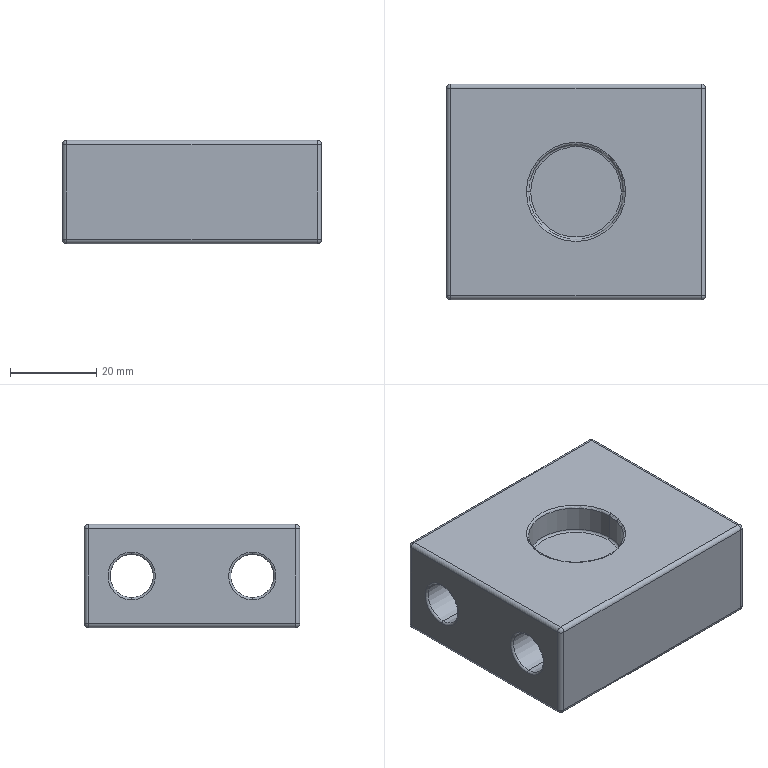Part | SolidWorks | features Fillet 2, ICE 2, Extrusion 1 | 1 solid | 45 faces | box 60 x 50 x 24 mm | volume 59794 mm3 | cylinder 18 | torus 12 | sphere 8 | plane 7 | commonest cylinder face diameters 2 x12 10 x4 22 x2
STEP:
#1=CARTESIAN_POINT('',(-29.5,14.,5.));
#2=VERTEX_POINT('',#1);
#3=CARTESIAN_POINT('',(-29.5,14.,-5.));
#4=VERTEX_POINT('',#3);
#5=CARTESIAN_POINT('',(-29.5,14.,0.));
#6=DIRECTION('',(-1.,0.,0.));
#7=DIRECTION('',(0.,0.,-1.));
#8=AXIS2_PLACEMENT_3D('',#5,#6,#7);
#9=CIRCLE('',#8,5.);
#10=EDGE_CURVE('',#2,#4,#9,.T.);
#11=ORIENTED_EDGE('',*,*,#10,.F.);
#12=CARTESIAN_POINT('',(-30.,14.,5.5));
#13=VERTEX_POINT('',#12);
#14=CARTESIAN_POINT('',(-29.5,14.,5.5));
#15=DIRECTION('',(0.,1.,0.));
#16=DIRECTION('',(0.,0.,1.));
#17=AXIS2_PLACEMENT_3D('',#14,#15,#16);
#18=CIRCLE('',#17,0.5);
#19=EDGE_CURVE('',#2,#13,#18,.T.);
#20=ORIENTED_EDGE('',*,*,#19,.T.);
#21=CARTESIAN_POINT('',(-30.,14.,-5.5));
#22=VERTEX_POINT('',#21);
#23=CARTESIAN_POINT('',(-30.,14.,0.));
#24=DIRECTION('',(1.,0.,0.));
#25=DIRECTION('',(0.,0.,-1.));
#26=AXIS2_PLACEMENT_3D('',#23,#24,#25);
#27=CIRCLE('',#26,5.5);
#28=EDGE_CURVE('',#22,#13,#27,.T.);
#29=ORIENTED_EDGE('',*,*,#28,.F.);
#30=CARTESIAN_POINT('',(-29.5,14.,-5.5));
#31=DIRECTION('',(0.,-1.,0.));
#32=DIRECTION('',(0.,0.,-1.));
#33=AXIS2_PLACEMENT_3D('',#30,#31,#32);
#34=CIRCLE('',#33,0.5);
#35=EDGE_CURVE('',#4,#22,#34,.T.);
#36=ORIENTED_EDGE('',*,*,#35,.F.);
#37=EDGE_LOOP('',(#11,#20,#29,#36));
#38=FACE_OUTER_BOUND('',#37,.T.);
#39=CARTESIAN_POINT('',(-29.5,14.,0.));
#40=DIRECTION('',(1.,0.,0.));
#41=DIRECTION('',(0.,0.,-1.));
#42=AXIS2_PLACEMENT_3D('',#39,#40,#41);
#43=TOROIDAL_SURFACE('',#42,5.5,0.5);
#44=ADVANCED_FACE('',(#38),#43,.T.);
#45=CARTESIAN_POINT('',(29.5,14.,-5.));
#46=VERTEX_POINT('',#45);
#47=CARTESIAN_POINT('',(29.5,14.,5.));
#48=VERTEX_POINT('',#47);
#49=CARTESIAN_POINT('',(29.5,14.,0.));
#50=DIRECTION('',(1.,0.,0.));
#51=DIRECTION('',(0.,0.,1.));
#52=AXIS2_PLACEMENT_3D('',#49,#50,#51);
#53=CIRCLE('',#52,5.);
#54=EDGE_CURVE('',#46,#48,#53,.T.);
#55=ORIENTED_EDGE('',*,*,#54,.F.);
#56=CARTESIAN_POINT('',(30.,14.,-5.5));
#57=VERTEX_POINT('',#56);
#58=CARTESIAN_POINT('',(29.5,14.,-5.5));
#59=DIRECTION('',(0.,1.,0.));
#60=DIRECTION('',(0.,0.,1.));
#61=AXIS2_PLACEMENT_3D('',#58,#59,#60);
#62=CIRCLE('',#61,0.5);
#63=EDGE_CURVE('',#46,#57,#62,.T.);
#64=ORIENTED_EDGE('',*,*,#63,.T.);
#65=CARTESIAN_POINT('',(30.,14.,5.5));
#66=VERTEX_POINT('',#65);
#67=CARTESIAN_POINT('',(30.,14.,0.));
#68=DIRECTION('',(-1.,0.,0.));
#69=DIRECTION('',(0.,0.,1.));
#70=AXIS2_PLACEMENT_3D('',#67,#68,#69);
#71=CIRCLE('',#70,5.5);
#72=EDGE_CURVE('',#66,#57,#71,.T.);
#73=ORIENTED_EDGE('',*,*,#72,.F.);
#74=CARTESIAN_POINT('',(29.5,14.,5.5));
#75=DIRECTION('',(0.,-1.,0.));
#76=DIRECTION('',(0.,0.,-1.));
#77=AXIS2_PLACEMENT_3D('',#74,#75,#76);
#78=CIRCLE('',#77,0.5);
#79=EDGE_CURVE('',#48,#66,#78,.T.);
#80=ORIENTED_EDGE('',*,*,#79,.F.);
#81=EDGE_LOOP('',(#55,#64,#73,#80));
#82=FACE_OUTER_BOUND('',#81,.T.);
#83=CARTESIAN_POINT('',(29.5,14.,0.));
#84=DIRECTION('',(-1.,0.,0.));
#85=DIRECTION('',(0.,0.,1.));
#86=AXIS2_PLACEMENT_3D('',#83,#84,#85);
#87=TOROIDAL_SURFACE('',#86,5.5,0.5);
#88=ADVANCED_FACE('',(#82),#87,.T.);
#89=CARTESIAN_POINT('',(-29.5,-14.,5.));
#90=VERTEX_POINT('',#89);
#91=CARTESIAN_POINT('',(-29.5,-14.,-5.));
#92=VERTEX_POINT('',#91);
#93=CARTESIAN_POINT('',(-29.5,-14.,0.));
#94=DIRECTION('',(-1.,0.,0.));
#95=DIRECTION('',(0.,0.,-1.));
#96=AXIS2_PLACEMENT_3D('',#93,#94,#95);
#97=CIRCLE('',#96,5.);
#98=EDGE_CURVE('',#90,#92,#97,.T.);
#99=ORIENTED_EDGE('',*,*,#98,.F.);
#100=CARTESIAN_POINT('',(-30.,-14.,5.5));
#101=VERTEX_POINT('',#100);
#102=CARTESIAN_POINT('',(-29.5,-14.,5.5));
#103=DIRECTION('',(0.,1.,0.));
#104=DIRECTION('',(0.,0.,1.));
#105=AXIS2_PLACEMENT_3D('',#102,#103,#104);
#106=CIRCLE('',#105,0.5);
#107=EDGE_CURVE('',#90,#101,#106,.T.);
#108=ORIENTED_EDGE('',*,*,#107,.T.);
#109=CARTESIAN_POINT('',(-30.,-14.,-5.5));
#110=VERTEX_POINT('',#109);
#111=CARTESIAN_POINT('',(-30.,-14.,0.));
#112=DIRECTION('',(1.,0.,0.));
#113=DIRECTION('',(0.,0.,-1.));
#114=AXIS2_PLACEMENT_3D('',#111,#112,#113);
#115=CIRCLE('',#114,5.5);
#116=EDGE_CURVE('',#110,#101,#115,.T.);
#117=ORIENTED_EDGE('',*,*,#116,.F.);
#118=CARTESIAN_POINT('',(-29.5,-14.,-5.5));
#119=DIRECTION('',(0.,-1.,0.));
#120=DIRECTION('',(0.,0.,-1.));
#121=AXIS2_PLACEMENT_3D('',#118,#119,#120);
#122=CIRCLE('',#121,0.5);
#123=EDGE_CURVE('',#92,#110,#122,.T.);
#124=ORIENTED_EDGE('',*,*,#123,.F.);
#125=EDGE_LOOP('',(#99,#108,#117,#124));
#126=FACE_OUTER_BOUND('',#125,.T.);
#127=CARTESIAN_POINT('',(-29.5,-14.,0.));
#128=DIRECTION('',(1.,0.,0.));
#129=DIRECTION('',(0.,0.,-1.));
#130=AXIS2_PLACEMENT_3D('',#127,#128,#129);
#131=TOROIDAL_SURFACE('',#130,5.5,0.5);
#132=ADVANCED_FACE('',(#126),#131,.T.);
#133=CARTESIAN_POINT('',(29.5,-14.,-5.));
#134=VERTEX_POINT('',#133);
#135=CARTESIAN_POINT('',(29.5,-14.,5.));
#136=VERTEX_POINT('',#135);
#137=CARTESIAN_POINT('',(29.5,-14.,0.));
#138=DIRECTION('',(1.,0.,0.));
#139=DIRECTION('',(0.,0.,1.));
#140=AXIS2_PLACEMENT_3D('',#137,#138,#139);
#141=CIRCLE('',#140,5.);
#142=EDGE_CURVE('',#134,#136,#141,.T.);
#143=ORIENTED_EDGE('',*,*,#142,.F.);
#144=CARTESIAN_POINT('',(30.,-14.,-5.5));
#145=VERTEX_POINT('',#144);
#146=CARTESIAN_POINT('',(29.5,-14.,-5.5));
#147=DIRECTION('',(0.,1.,0.));
#148=DIRECTION('',(0.,0.,1.));
#149=AXIS2_PLACEMENT_3D('',#146,#147,#148);
#150=CIRCLE('',#149,0.5);
#151=EDGE_CURVE('',#134,#145,#150,.T.);
#152=ORIENTED_EDGE('',*,*,#151,.T.);
#153=CARTESIAN_POINT('',(30.,-14.,5.5));
#154=VERTEX_POINT('',#153);
#155=CARTESIAN_POINT('',(30.,-14.,0.));
#156=DIRECTION('',(-1.,0.,0.));
#157=DIRECTION('',(0.,0.,1.));
#158=AXIS2_PLACEMENT_3D('',#155,#156,#157);
#159=CIRCLE('',#158,5.5);
#160=EDGE_CURVE('',#154,#145,#159,.T.);
#161=ORIENTED_EDGE('',*,*,#160,.F.);
#162=CARTESIAN_POINT('',(29.5,-14.,5.5));
#163=DIRECTION('',(0.,-1.,0.));
#164=DIRECTION('',(0.,0.,-1.));
#165=AXIS2_PLACEMENT_3D('',#162,#163,#164);
#166=CIRCLE('',#165,0.5);
#167=EDGE_CURVE('',#136,#154,#166,.T.);
#168=ORIENTED_EDGE('',*,*,#167,.F.);
#169=EDGE_LOOP('',(#143,#152,#161,#168));
#170=FACE_OUTER_BOUND('',#169,.T.);
#171=CARTESIAN_POINT('',(29.5,-14.,0.));
#172=DIRECTION('',(-1.,0.,0.));
#173=DIRECTION('',(0.,0.,1.));
#174=AXIS2_PLACEMENT_3D('',#171,#172,#173);
#175=TOROIDAL_SURFACE('',#174,5.5,0.5);
#176=ADVANCED_FACE('',(#170),#175,.T.);
#177=CARTESIAN_POINT('',(-10.5,0.,5.));
#178=VERTEX_POINT('',#177);
#179=CARTESIAN_POINT('',(10.5,0.,5.));
#180=VERTEX_POINT('',#179);
#181=CARTESIAN_POINT('',(0.,0.,5.));
#182=DIRECTION('',(0.,0.,1.));
#183=DIRECTION('',(1.,0.,0.));
#184=AXIS2_PLACEMENT_3D('',#181,#182,#183);
#185=CIRCLE('',#184,10.5);
#186=EDGE_CURVE('',#178,#180,#185,.T.);
#187=ORIENTED_EDGE('',*,*,#186,.F.);
#188=CARTESIAN_POINT('',(-11.,0.,5.5));
#189=VERTEX_POINT('',#188);
#190=CARTESIAN_POINT('',(-10.5,0.,5.5));
#191=DIRECTION('',(0.,1.,0.));
#192=DIRECTION('',(-1.,0.,0.));
#193=AXIS2_PLACEMENT_3D('',#190,#191,#192);
#194=CIRCLE('',#193,0.5);
#195=EDGE_CURVE('',#178,#189,#194,.T.);
#196=ORIENTED_EDGE('',*,*,#195,.T.);
#197=CARTESIAN_POINT('',(11.,0.,5.5));
#198=VERTEX_POINT('',#197);
#199=CARTESIAN_POINT('',(0.,0.,5.5));
#200=DIRECTION('',(0.,0.,-1.));
#201=DIRECTION('',(1.,0.,0.));
#202=AXIS2_PLACEMENT_3D('',#199,#200,#201);
#203=CIRCLE('',#202,11.);
#204=EDGE_CURVE('',#198,#189,#203,.T.);
#205=ORIENTED_EDGE('',*,*,#204,.F.);
#206=CARTESIAN_POINT('',(10.5,0.,5.5));
#207=DIRECTION('',(0.,-1.,0.));
#208=DIRECTION('',(0.,0.,-1.));
#209=AXIS2_PLACEMENT_3D('',#206,#207,#208);
#210=CIRCLE('',#209,0.5);
#211=EDGE_CURVE('',#180,#198,#210,.T.);
#212=ORIENTED_EDGE('',*,*,#211,.F.);
#213=EDGE_LOOP('',(#187,#196,#205,#212));
#214=FACE_OUTER_BOUND('',#213,.T.);
#215=CARTESIAN_POINT('',(0.,0.,5.5));
#216=DIRECTION('',(0.,0.,1.));
#217=DIRECTION('',(1.,0.,0.));
#218=AXIS2_PLACEMENT_3D('',#215,#216,#217);
#219=TOROIDAL_SURFACE('',#218,10.5,0.5);
#220=ADVANCED_FACE('',(#214),#219,.F.);
#221=CARTESIAN_POINT('',(-11.5,0.,12.));
#222=VERTEX_POINT('',#221);
#223=CARTESIAN_POINT('',(11.5,0.,12.));
#224=VERTEX_POINT('',#223);
#225=CARTESIAN_POINT('',(0.,0.,12.));
#226=DIRECTION('',(0.,0.,-1.));
#227=DIRECTION('',(1.,0.,0.));
#228=AXIS2_PLACEMENT_3D('',#225,#226,#227);
#229=CIRCLE('',#228,11.5);
#230=EDGE_CURVE('',#222,#224,#229,.T.);
#231=ORIENTED_EDGE('',*,*,#230,.F.);
#232=CARTESIAN_POINT('',(-11.,0.,11.5));
#233=VERTEX_POINT('',#232);
#234=CARTESIAN_POINT('',(-11.5,0.,11.5));
#235=DIRECTION('',(0.,1.,0.));
#236=DIRECTION('',(-1.,0.,0.));
#237=AXIS2_PLACEMENT_3D('',#234,#235,#236);
#238=CIRCLE('',#237,0.5);
#239=EDGE_CURVE('',#222,#233,#238,.T.);
#240=ORIENTED_EDGE('',*,*,#239,.T.);
#241=CARTESIAN_POINT('',(11.,0.,11.5));
#242=VERTEX_POINT('',#241);
#243=CARTESIAN_POINT('',(0.,0.,11.5));
#244=DIRECTION('',(0.,0.,1.));
#245=DIRECTION('',(1.,0.,0.));
#246=AXIS2_PLACEMENT_3D('',#243,#244,#245);
#247=CIRCLE('',#246,11.);
#248=EDGE_CURVE('',#242,#233,#247,.T.);
#249=ORIENTED_EDGE('',*,*,#248,.F.);
#250=CARTESIAN_POINT('',(11.5,0.,11.5));
#251=DIRECTION('',(0.,-1.,0.));
#252=DIRECTION('',(0.,0.,-1.));
#253=AXIS2_PLACEMENT_3D('',#250,#251,#252);
#254=CIRCLE('',#253,0.5);
#255=EDGE_CURVE('',#224,#242,#254,.T.);
#256=ORIENTED_EDGE('',*,*,#255,.F.);
#257=EDGE_LOOP('',(#231,#240,#249,#256));
#258=FACE_OUTER_BOUND('',#257,.T.);
#259=CARTESIAN_POINT('',(0.,0.,11.5));
#260=DIRECTION('',(0.,0.,1.));
#261=DIRECTION('',(1.,0.,0.));
#262=AXIS2_PLACEMENT_3D('',#259,#260,#261);
#263=TOROIDAL_SURFACE('',#262,11.5,0.5);
#264=ADVANCED_FACE('',(#258),#263,.T.);
#265=CARTESIAN_POINT('',(-29.5,-14.,0.));
#266=DIRECTION('',(-1.,0.,0.));
#267=DIRECTION('',(0.,0.,-1.));
#268=AXIS2_PLACEMENT_3D('',#265,#266,#267);
#269=CIRCLE('',#268,5.);
#270=EDGE_CURVE('',#92,#90,#269,.T.);
#271=ORIENTED_EDGE('',*,*,#270,.T.);
#272=CARTESIAN_POINT('',(-30.,-14.,5.));
#273=DIRECTION('',(1.,0.,0.));
#274=VECTOR('',#273,1000.);
#275=LINE('',#272,#274);
#276=EDGE_CURVE('',#90,#136,#275,.T.);
#277=ORIENTED_EDGE('',*,*,#276,.T.);
#278=CARTESIAN_POINT('',(29.5,-14.,0.));
#279=DIRECTION('',(1.,0.,0.));
#280=DIRECTION('',(0.,0.,1.));
#281=AXIS2_PLACEMENT_3D('',#278,#279,#280);
#282=CIRCLE('',#281,5.);
#283=EDGE_CURVE('',#136,#134,#282,.T.);
#284=ORIENTED_EDGE('',*,*,#283,.T.);
#285=CARTESIAN_POINT('',(-30.,-14.,-5.));
#286=DIRECTION('',(1.,0.,0.));
#287=VECTOR('',#286,1000.);
#288=LINE('',#285,#287);
#289=EDGE_CURVE('',#92,#134,#288,.T.);
#290=ORIENTED_EDGE('',*,*,#289,.F.);
#291=EDGE_LOOP('',(#271,#277,#284,#290));
#292=FACE_OUTER_BOUND('',#291,.T.);
#293=CARTESIAN_POINT('',(-30.,-14.,0.));
#294=DIRECTION('',(1.,0.,0.));
#295=DIRECTION('',(0.,0.,-1.));
#296=AXIS2_PLACEMENT_3D('',#293,#294,#295);
#297=CYLINDRICAL_SURFACE('',#296,5.);
#298=ADVANCED_FACE('',(#292),#297,.F.);
#299=CARTESIAN_POINT('',(-29.5,14.,0.));
#300=DIRECTION('',(-1.,0.,0.));
#301=DIRECTION('',(0.,0.,-1.));
#302=AXIS2_PLACEMENT_3D('',#299,#300,#301);
#303=CIRCLE('',#302,5.);
#304=EDGE_CURVE('',#4,#2,#303,.T.);
#305=ORIENTED_EDGE('',*,*,#304,.T.);
#306=CARTESIAN_POINT('',(-30.,14.,5.));
#307=DIRECTION('',(1.,0.,0.));
#308=VECTOR('',#307,1000.);
#309=LINE('',#306,#308);
#310=EDGE_CURVE('',#2,#48,#309,.T.);
#311=ORIENTED_EDGE('',*,*,#310,.T.);
#312=CARTESIAN_POINT('',(29.5,14.,0.));
#313=DIRECTION('',(1.,0.,0.));
#314=DIRECTION('',(0.,0.,1.));
#315=AXIS2_PLACEMENT_3D('',#312,#313,#314);
#316=CIRCLE('',#315,5.);
#317=EDGE_CURVE('',#48,#46,#316,.T.);
#318=ORIENTED_EDGE('',*,*,#317,.T.);
#319=CARTESIAN_POINT('',(-30.,14.,-5.));
#320=DIRECTION('',(1.,0.,0.));
#321=VECTOR('',#320,1000.);
#322=LINE('',#319,#321);
#323=EDGE_CURVE('',#4,#46,#322,.T.);
#324=ORIENTED_EDGE('',*,*,#323,.F.);
#325=EDGE_LOOP('',(#305,#311,#318,#324));
#326=FACE_OUTER_BOUND('',#325,.T.);
#327=CARTESIAN_POINT('',(-30.,14.,0.));
#328=DIRECTION('',(1.,0.,0.));
#329=DIRECTION('',(0.,0.,-1.));
#330=AXIS2_PLACEMENT_3D('',#327,#328,#329);
#331=CYLINDRICAL_SURFACE('',#330,5.);
#332=ADVANCED_FACE('',(#326),#331,.F.);
#333=ORIENTED_EDGE('',*,*,#204,.T.);
#334=CARTESIAN_POINT('',(-11.,0.,5.));
#335=DIRECTION('',(0.,0.,1.));
#336=VECTOR('',#335,1000.);
#337=LINE('',#334,#336);
#338=EDGE_CURVE('',#189,#233,#337,.T.);
#339=ORIENTED_EDGE('',*,*,#338,.T.);
#340=CARTESIAN_POINT('',(0.,0.,11.5));
#341=DIRECTION('',(0.,0.,1.));
#342=DIRECTION('',(1.,0.,0.));
#343=AXIS2_PLACEMENT_3D('',#340,#341,#342);
#344=CIRCLE('',#343,11.);
#345=EDGE_CURVE('',#233,#242,#344,.T.);
#346=ORIENTED_EDGE('',*,*,#345,.T.);
#347=CARTESIAN_POINT('',(11.,0.,5.));
#348=DIRECTION('',(0.,0.,1.));
#349=VECTOR('',#348,1000.);
#350=LINE('',#347,#349);
#351=EDGE_CURVE('',#198,#242,#350,.T.);
#352=ORIENTED_EDGE('',*,*,#351,.F.);
#353=EDGE_LOOP('',(#333,#339,#346,#352));
#354=FACE_OUTER_BOUND('',#353,.T.);
#355=CARTESIAN_POINT('',(0.,0.,5.));
#356=DIRECTION('',(0.,0.,1.));
#357=DIRECTION('',(1.,0.,0.));
#358=AXIS2_PLACEMENT_3D('',#355,#356,#357);
#359=CYLINDRICAL_SURFACE('',#358,11.);
#360=ADVANCED_FACE('',(#354),#359,.F.);
#361=ORIENTED_EDGE('',*,*,#116,.T.);
#362=CARTESIAN_POINT('',(-30.,-14.,0.));
#363=DIRECTION('',(1.,0.,0.));
#364=DIRECTION('',(0.,0.,-1.));
#365=AXIS2_PLACEMENT_3D('',#362,#363,#364);
#366=CIRCLE('',#365,5.5);
#367=EDGE_CURVE('',#101,#110,#366,.T.);
#368=ORIENTED_EDGE('',*,*,#367,.T.);
#369=EDGE_LOOP('',(#361,#368));
#370=FACE_BOUND('',#369,.T.);
#371=ORIENTED_EDGE('',*,*,#28,.T.);
#372=CARTESIAN_POINT('',(-30.,14.,0.));
#373=DIRECTION('',(1.,0.,0.));
#374=DIRECTION('',(0.,0.,-1.));
#375=AXIS2_PLACEMENT_3D('',#372,#373,#374);
#376=CIRCLE('',#375,5.5);
#377=EDGE_CURVE('',#13,#22,#376,.T.);
#378=ORIENTED_EDGE('',*,*,#377,.T.);
#379=EDGE_LOOP('',(#371,#378));
#380=FACE_BOUND('',#379,.T.);
#381=CARTESIAN_POINT('',(-30.,24.,11.));
#382=VERTEX_POINT('',#381);
#383=CARTESIAN_POINT('',(-30.,24.,-11.));
#384=VERTEX_POINT('',#383);
#385=CARTESIAN_POINT('',(-30.,24.,12.));
#386=DIRECTION('',(0.,0.,-1.));
#387=VECTOR('',#386,1000.);
#388=LINE('',#385,#387);
#389=EDGE_CURVE('',#382,#384,#388,.T.);
#390=ORIENTED_EDGE('',*,*,#389,.T.);
#391=CARTESIAN_POINT('',(-30.,-24.,-11.));
#392=VERTEX_POINT('',#391);
#393=CARTESIAN_POINT('',(-30.,-25.,-11.));
#394=DIRECTION('',(0.,-1.,0.));
#395=VECTOR('',#394,1000.);
#396=LINE('',#393,#395);
#397=EDGE_CURVE('',#384,#392,#396,.T.);
#398=ORIENTED_EDGE('',*,*,#397,.T.);
#399=CARTESIAN_POINT('',(-30.,-24.,11.));
#400=VERTEX_POINT('',#399);
#401=CARTESIAN_POINT('',(-30.,-24.,12.));
#402=DIRECTION('',(0.,0.,1.));
#403=VECTOR('',#402,1000.);
#404=LINE('',#401,#403);
#405=EDGE_CURVE('',#392,#400,#404,.T.);
#406=ORIENTED_EDGE('',*,*,#405,.T.);
#407=CARTESIAN_POINT('',(-30.,25.,11.));
#408=DIRECTION('',(0.,1.,0.));
#409=VECTOR('',#408,1000.);
#410=LINE('',#407,#409);
#411=EDGE_CURVE('',#400,#382,#410,.T.);
#412=ORIENTED_EDGE('',*,*,#411,.T.);
#413=EDGE_LOOP('',(#390,#398,#406,#412));
#414=FACE_OUTER_BOUND('',#413,.T.);
#415=CARTESIAN_POINT('',(-30.,-25.,12.));
#416=DIRECTION('',(1.,0.,0.));
#417=DIRECTION('',(0.,0.,-1.));
#418=AXIS2_PLACEMENT_3D('',#415,#416,#417);
#419=PLANE('',#418);
#420=ADVANCED_FACE('',(#370,#380,#414),#419,.F.);
#421=CARTESIAN_POINT('',(29.,-25.,11.));
#422=VERTEX_POINT('',#421);
#423=CARTESIAN_POINT('',(-29.,-25.,11.));
#424=VERTEX_POINT('',#423);
#425=CARTESIAN_POINT('',(-30.,-25.,11.));
#426=DIRECTION('',(-1.,0.,0.));
#427=VECTOR('',#426,1000.);
#428=LINE('',#425,#427);
#429=EDGE_CURVE('',#422,#424,#428,.T.);
#430=ORIENTED_EDGE('',*,*,#429,.T.);
#431=CARTESIAN_POINT('',(-29.,-25.,-11.));
#432=VERTEX_POINT('',#431);
#433=CARTESIAN_POINT('',(-29.,-25.,12.));
#434=DIRECTION('',(0.,0.,-1.));
#435=VECTOR('',#434,1000.);
#436=LINE('',#433,#435);
#437=EDGE_CURVE('',#424,#432,#436,.T.);
#438=ORIENTED_EDGE('',*,*,#437,.T.);
#439=CARTESIAN_POINT('',(29.,-25.,-11.));
#440=VERTEX_POINT('',#439);
#441=CARTESIAN_POINT('',(30.,-25.,-11.));
#442=DIRECTION('',(1.,0.,0.));
#443=VECTOR('',#442,1000.);
#444=LINE('',#441,#443);
#445=EDGE_CURVE('',#432,#440,#444,.T.);
#446=ORIENTED_EDGE('',*,*,#445,.T.);
#447=CARTESIAN_POINT('',(29.,-25.,12.));
#448=DIRECTION('',(0.,0.,1.));
#449=VECTOR('',#448,1000.);
#450=LINE('',#447,#449);
#451=EDGE_CURVE('',#440,#422,#450,.T.);
#452=ORIENTED_EDGE('',*,*,#451,.T.);
#453=EDGE_LOOP('',(#430,#438,#446,#452));
#454=FACE_OUTER_BOUND('',#453,.T.);
#455=CARTESIAN_POINT('',(30.,-25.,12.));
#456=DIRECTION('',(0.,1.,0.));
#457=DIRECTION('',(-1.,0.,0.));
#458=AXIS2_PLACEMENT_3D('',#455,#456,#457);
#459=PLANE('',#458);
#460=ADVANCED_FACE('',(#454),#459,.F.);
#461=ORIENTED_EDGE('',*,*,#160,.T.);
#462=CARTESIAN_POINT('',(30.,-14.,0.));
#463=DIRECTION('',(-1.,0.,0.));
#464=DIRECTION('',(0.,0.,1.));
#465=AXIS2_PLACEMENT_3D('',#462,#463,#464);
#466=CIRCLE('',#465,5.5);
#467=EDGE_CURVE('',#145,#154,#466,.T.);
#468=ORIENTED_EDGE('',*,*,#467,.T.);
#469=EDGE_LOOP('',(#461,#468));
#470=FACE_BOUND('',#469,.T.);
#471=ORIENTED_EDGE('',*,*,#72,.T.);
#472=CARTESIAN_POINT('',(30.,14.,0.));
#473=DIRECTION('',(-1.,0.,0.));
#474=DIRECTION('',(0.,0.,1.));
#475=AXIS2_PLACEMENT_3D('',#472,#473,#474);
#476=CIRCLE('',#475,5.5);
#477=EDGE_CURVE('',#57,#66,#476,.T.);
#478=ORIENTED_EDGE('',*,*,#477,.T.);
#479=EDGE_LOOP('',(#471,#478));
#480=FACE_BOUND('',#479,.T.);
#481=CARTESIAN_POINT('',(30.,-24.,11.));
#482=VERTEX_POINT('',#481);
#483=CARTESIAN_POINT('',(30.,-24.,-11.));
#484=VERTEX_POINT('',#483);
#485=CARTESIAN_POINT('',(30.,-24.,12.));
#486=DIRECTION('',(0.,0.,-1.));
#487=VECTOR('',#486,1000.);
#488=LINE('',#485,#487);
#489=EDGE_CURVE('',#482,#484,#488,.T.);
#490=ORIENTED_EDGE('',*,*,#489,.T.);
#491=CARTESIAN_POINT('',(30.,24.,-11.));
#492=VERTEX_POINT('',#491);
#493=CARTESIAN_POINT('',(30.,-25.,-11.));
#494=DIRECTION('',(0.,1.,0.));
#495=VECTOR('',#494,1000.);
#496=LINE('',#493,#495);
#497=EDGE_CURVE('',#484,#492,#496,.T.);
#498=ORIENTED_EDGE('',*,*,#497,.T.);
#499=CARTESIAN_POINT('',(30.,24.,11.));
#500=VERTEX_POINT('',#499);
#501=CARTESIAN_POINT('',(30.,24.,12.));
#502=DIRECTION('',(0.,0.,1.));
#503=VECTOR('',#502,1000.);
#504=LINE('',#501,#503);
#505=EDGE_CURVE('',#492,#500,#504,.T.);
#506=ORIENTED_EDGE('',*,*,#505,.T.);
#507=CARTESIAN_POINT('',(30.,-25.,11.));
#508=DIRECTION('',(0.,-1.,0.));
#509=VECTOR('',#508,1000.);
#510=LINE('',#507,#509);
#511=EDGE_CURVE('',#500,#482,#510,.T.);
#512=ORIENTED_EDGE('',*,*,#511,.T.);
#513=EDGE_LOOP('',(#490,#498,#506,#512));
#514=FACE_OUTER_BOUND('',#513,.T.);
#515=CARTESIAN_POINT('',(30.,-25.,12.));
#516=DIRECTION('',(-1.,0.,0.));
#517=DIRECTION('',(0.,0.,1.));
#518=AXIS2_PLACEMENT_3D('',#515,#516,#517);
#519=PLANE('',#518);
#520=ADVANCED_FACE('',(#470,#480,#514),#519,.F.);
#521=CARTESIAN_POINT('',(-29.,25.,11.));
#522=VERTEX_POINT('',#521);
#523=CARTESIAN_POINT('',(29.,25.,11.));
#524=VERTEX_POINT('',#523);
#525=CARTESIAN_POINT('',(30.,25.,11.));
#526=DIRECTION('',(1.,0.,0.));
#527=VECTOR('',#526,1000.);
#528=LINE('',#525,#527);
#529=EDGE_CURVE('',#522,#524,#528,.T.);
#530=ORIENTED_EDGE('',*,*,#529,.T.);
#531=CARTESIAN_POINT('',(29.,25.,-11.));
#532=VERTEX_POINT('',#531);
#533=CARTESIAN_POINT('',(29.,25.,12.));
#534=DIRECTION('',(0.,0.,-1.));
#535=VECTOR('',#534,1000.);
#536=LINE('',#533,#535);
#537=EDGE_CURVE('',#524,#532,#536,.T.);
#538=ORIENTED_EDGE('',*,*,#537,.T.);
#539=CARTESIAN_POINT('',(-29.,25.,-11.));
#540=VERTEX_POINT('',#539);
#541=CARTESIAN_POINT('',(30.,25.,-11.));
#542=DIRECTION('',(-1.,0.,0.));
#543=VECTOR('',#542,1000.);
#544=LINE('',#541,#543);
#545=EDGE_CURVE('',#532,#540,#544,.T.);
#546=ORIENTED_EDGE('',*,*,#545,.T.);
#547=CARTESIAN_POINT('',(-29.,25.,12.));
#548=DIRECTION('',(0.,0.,1.));
#549=VECTOR('',#548,1000.);
#550=LINE('',#547,#549);
#551=EDGE_CURVE('',#540,#522,#550,.T.);
#552=ORIENTED_EDGE('',*,*,#551,.T.);
#553=EDGE_LOOP('',(#530,#538,#546,#552));
#554=FACE_OUTER_BOUND('',#553,.T.);
#555=CARTESIAN_POINT('',(30.,25.,12.));
#556=DIRECTION('',(0.,-1.,0.));
#557=DIRECTION('',(1.,0.,0.));
#558=AXIS2_PLACEMENT_3D('',#555,#556,#557);
#559=PLANE('',#558);
#560=ADVANCED_FACE('',(#554),#559,.F.);
#561=CARTESIAN_POINT('',(0.,0.,12.));
#562=DIRECTION('',(0.,0.,-1.));
#563=DIRECTION('',(1.,0.,0.));
#564=AXIS2_PLACEMENT_3D('',#561,#562,#563);
#565=CIRCLE('',#564,11.5);
#566=EDGE_CURVE('',#224,#222,#565,.T.);
#567=ORIENTED_EDGE('',*,*,#566,.T.);
#568=ORIENTED_EDGE('',*,*,#230,.T.);
#569=EDGE_LOOP('',(#567,#568));
#570=FACE_BOUND('',#569,.T.);
#571=CARTESIAN_POINT('',(29.,24.,12.));
#572=VERTEX_POINT('',#571);
#573=CARTESIAN_POINT('',(-29.,24.,12.));
#574=VERTEX_POINT('',#573);
#575=CARTESIAN_POINT('',(-30.,24.,12.));
#576=DIRECTION('',(-1.,0.,0.));
#577=VECTOR('',#576,1000.);
#578=LINE('',#575,#577);
#579=EDGE_CURVE('',#572,#574,#578,.T.);
#580=ORIENTED_EDGE('',*,*,#579,.T.);
#581=CARTESIAN_POINT('',(-29.,-24.,12.));
#582=VERTEX_POINT('',#581);
#583=CARTESIAN_POINT('',(-29.,-25.,12.));
#584=DIRECTION('',(0.,-1.,0.));
#585=VECTOR('',#584,1000.);
#586=LINE('',#583,#585);
#587=EDGE_CURVE('',#574,#582,#586,.T.);
#588=ORIENTED_EDGE('',*,*,#587,.T.);
#589=CARTESIAN_POINT('',(29.,-24.,12.));
#590=VERTEX_POINT('',#589);
#591=CARTESIAN_POINT('',(30.,-24.,12.));
#592=DIRECTION('',(1.,0.,0.));
#593=VECTOR('',#592,1000.);
#594=LINE('',#591,#593);
#595=EDGE_CURVE('',#582,#590,#594,.T.);
#596=ORIENTED_EDGE('',*,*,#595,.T.);
#597=CARTESIAN_POINT('',(29.,25.,12.));
#598=DIRECTION('',(0.,1.,0.));
#599=VECTOR('',#598,1000.);
#600=LINE('',#597,#599);
#601=EDGE_CURVE('',#590,#572,#600,.T.);
#602=ORIENTED_EDGE('',*,*,#601,.T.);
#603=EDGE_LOOP('',(#580,#588,#596,#602));
#604=FACE_OUTER_BOUND('',#603,.T.);
#605=CARTESIAN_POINT('',(0.,0.,12.));
#606=DIRECTION('',(0.,0.,1.));
#607=DIRECTION('',(1.,0.,0.));
#608=AXIS2_PLACEMENT_3D('',#605,#606,#607);
#609=PLANE('',#608);
#610=ADVANCED_FACE('',(#570,#604),#609,.T.);
#611=CARTESIAN_POINT('',(29.,-24.,-12.));
#612=VERTEX_POINT('',#611);
#613=CARTESIAN_POINT('',(-29.,-24.,-12.));
#614=VERTEX_POINT('',#613);
#615=CARTESIAN_POINT('',(0.,-24.,-12.));
#616=DIRECTION('',(-1.,0.,0.));
#617=VECTOR('',#616,1000.);
#618=LINE('',#615,#617);
#619=EDGE_CURVE('',#612,#614,#618,.T.);
#620=ORIENTED_EDGE('',*,*,#619,.T.);
#621=CARTESIAN_POINT('',(-29.,24.,-12.));
#622=VERTEX_POINT('',#621);
#623=CARTESIAN_POINT('',(-29.,0.,-12.));
#624=DIRECTION('',(0.,1.,0.));
#625=VECTOR('',#624,1000.);
#626=LINE('',#623,#625);
#627=EDGE_CURVE('',#614,#622,#626,.T.);
#628=ORIENTED_EDGE('',*,*,#627,.T.);
#629=CARTESIAN_POINT('',(29.,24.,-12.));
#630=VERTEX_POINT('',#629);
#631=CARTESIAN_POINT('',(0.,24.,-12.));
#632=DIRECTION('',(1.,0.,0.));
#633=VECTOR('',#632,1000.);
#634=LINE('',#631,#633);
#635=EDGE_CURVE('',#622,#630,#634,.T.);
#636=ORIENTED_EDGE('',*,*,#635,.T.);
#637=CARTESIAN_POINT('',(29.,0.,-12.));
#638=DIRECTION('',(0.,-1.,0.));
#639=VECTOR('',#638,1000.);
#640=LINE('',#637,#639);
#641=EDGE_CURVE('',#630,#612,#640,.T.);
#642=ORIENTED_EDGE('',*,*,#641,.T.);
#643=EDGE_LOOP('',(#620,#628,#636,#642));
#644=FACE_OUTER_BOUND('',#643,.T.);
#645=CARTESIAN_POINT('',(0.,0.,-12.));
#646=DIRECTION('',(0.,0.,1.));
#647=DIRECTION('',(1.,0.,0.));
#648=AXIS2_PLACEMENT_3D('',#645,#646,#647);
#649=PLANE('',#648);
#650=ADVANCED_FACE('',(#644),#649,.F.);
#651=ORIENTED_EDGE('',*,*,#338,.F.);
#652=CARTESIAN_POINT('',(0.,0.,5.5));
#653=DIRECTION('',(0.,0.,-1.));
#654=DIRECTION('',(1.,0.,0.));
#655=AXIS2_PLACEMENT_3D('',#652,#653,#654);
#656=CIRCLE('',#655,11.);
#657=EDGE_CURVE('',#189,#198,#656,.T.);
#658=ORIENTED_EDGE('',*,*,#657,.T.);
#659=ORIENTED_EDGE('',*,*,#351,.T.);
#660=ORIENTED_EDGE('',*,*,#248,.T.);
#661=EDGE_LOOP('',(#651,#658,#659,#660));
#662=FACE_OUTER_BOUND('',#661,.T.);
#663=CARTESIAN_POINT('',(0.,0.,5.));
#664=DIRECTION('',(0.,0.,1.));
#665=DIRECTION('',(1.,0.,0.));
#666=AXIS2_PLACEMENT_3D('',#663,#664,#665);
#667=CYLINDRICAL_SURFACE('',#666,11.);
#668=ADVANCED_FACE('',(#662),#667,.F.);
#669=CARTESIAN_POINT('',(0.,0.,5.));
#670=DIRECTION('',(0.,0.,1.));
#671=DIRECTION('',(1.,0.,0.));
#672=AXIS2_PLACEMENT_3D('',#669,#670,#671);
#673=CIRCLE('',#672,10.5);
#674=EDGE_CURVE('',#180,#178,#673,.T.);
#675=ORIENTED_EDGE('',*,*,#674,.T.);
#676=ORIENTED_EDGE('',*,*,#186,.T.);
#677=EDGE_LOOP('',(#675,#676));
#678=FACE_OUTER_BOUND('',#677,.T.);
#679=CARTESIAN_POINT('',(0.,0.,5.));
#680=DIRECTION('',(0.,0.,1.));
#681=DIRECTION('',(1.,0.,0.));
#682=AXIS2_PLACEMENT_3D('',#679,#680,#681);
#683=PLANE('',#682);
#684=ADVANCED_FACE('',(#678),#683,.T.);
#685=ORIENTED_EDGE('',*,*,#310,.F.);
#686=ORIENTED_EDGE('',*,*,#10,.T.);
#687=ORIENTED_EDGE('',*,*,#323,.T.);
#688=ORIENTED_EDGE('',*,*,#54,.T.);
#689=EDGE_LOOP('',(#685,#686,#687,#688));
#690=FACE_OUTER_BOUND('',#689,.T.);
#691=CARTESIAN_POINT('',(-30.,14.,0.));
#692=DIRECTION('',(1.,0.,0.));
#693=DIRECTION('',(0.,0.,-1.));
#694=AXIS2_PLACEMENT_3D('',#691,#692,#693);
#695=CYLINDRICAL_SURFACE('',#694,5.);
#696=ADVANCED_FACE('',(#690),#695,.F.);
#697=ORIENTED_EDGE('',*,*,#276,.F.);
#698=ORIENTED_EDGE('',*,*,#98,.T.);
#699=ORIENTED_EDGE('',*,*,#289,.T.);
#700=ORIENTED_EDGE('',*,*,#142,.T.);
#701=EDGE_LOOP('',(#697,#698,#699,#700));
#702=FACE_OUTER_BOUND('',#701,.T.);
#703=CARTESIAN_POINT('',(-30.,-14.,0.));
#704=DIRECTION('',(1.,0.,0.));
#705=DIRECTION('',(0.,0.,-1.));
#706=AXIS2_PLACEMENT_3D('',#703,#704,#705);
#707=CYLINDRICAL_SURFACE('',#706,5.);
#708=ADVANCED_FACE('',(#702),#707,.F.);
#709=CARTESIAN_POINT('',(29.,24.,11.));
#710=DIRECTION('',(0.,0.,1.));
#711=DIRECTION('',(1.,0.,0.));
#712=AXIS2_PLACEMENT_3D('',#709,#710,#711);
#713=CIRCLE('',#712,1.);
#714=EDGE_CURVE('',#500,#524,#713,.T.);
#715=ORIENTED_EDGE('',*,*,#714,.F.);
#716=ORIENTED_EDGE('',*,*,#505,.F.);
#717=CARTESIAN_POINT('',(29.,24.,-11.));
#718=DIRECTION('',(0.,0.,-1.));
#719=DIRECTION('',(-1.,0.,0.));
#720=AXIS2_PLACEMENT_3D('',#717,#718,#719);
#721=CIRCLE('',#720,1.);
#722=EDGE_CURVE('',#532,#492,#721,.T.);
#723=ORIENTED_EDGE('',*,*,#722,.F.);
#724=ORIENTED_EDGE('',*,*,#537,.F.);
#725=EDGE_LOOP('',(#715,#716,#723,#724));
#726=FACE_OUTER_BOUND('',#725,.T.);
#727=CARTESIAN_POINT('',(29.,24.,12.));
#728=DIRECTION('',(0.,0.,-1.));
#729=DIRECTION('',(-1.,0.,0.));
#730=AXIS2_PLACEMENT_3D('',#727,#728,#729);
#731=CYLINDRICAL_SURFACE('',#730,1.);
#732=ADVANCED_FACE('',(#726),#731,.T.);
#733=CARTESIAN_POINT('',(29.,24.,11.));
#734=DIRECTION('',(0.,-1.,0.));
#735=DIRECTION('',(0.,0.,1.));
#736=AXIS2_PLACEMENT_3D('',#733,#734,#735);
#737=CIRCLE('',#736,1.);
#738=EDGE_CURVE('',#500,#572,#737,.T.);
#739=ORIENTED_EDGE('',*,*,#738,.F.);
#740=ORIENTED_EDGE('',*,*,#714,.T.);
#741=CARTESIAN_POINT('',(29.,24.,11.));
#742=DIRECTION('',(-1.,0.,0.));
#743=DIRECTION('',(0.,0.,-1.));
#744=AXIS2_PLACEMENT_3D('',#741,#742,#743);
#745=CIRCLE('',#744,1.);
#746=EDGE_CURVE('',#572,#524,#745,.T.);
#747=ORIENTED_EDGE('',*,*,#746,.F.);
#748=EDGE_LOOP('',(#739,#740,#747));
#749=FACE_OUTER_BOUND('',#748,.T.);
#750=CARTESIAN_POINT('',(29.,24.,11.));
#751=DIRECTION('',(0.,1.,0.));
#752=DIRECTION('',(1.,0.,0.));
#753=AXIS2_PLACEMENT_3D('',#750,#751,#752);
#754=SPHERICAL_SURFACE('',#753,1.);
#755=ADVANCED_FACE('',(#749),#754,.T.);
#756=CARTESIAN_POINT('',(29.,24.,-11.));
#757=DIRECTION('',(-1.,0.,0.));
#758=DIRECTION('',(0.,0.,-1.));
#759=AXIS2_PLACEMENT_3D('',#756,#757,#758);
#760=CIRCLE('',#759,1.);
#761=EDGE_CURVE('',#532,#630,#760,.T.);
#762=ORIENTED_EDGE('',*,*,#761,.F.);
#763=ORIENTED_EDGE('',*,*,#722,.T.);
#764=CARTESIAN_POINT('',(29.,24.,-11.));
#765=DIRECTION('',(0.,-1.,0.));
#766=DIRECTION('',(0.,0.,1.));
#767=AXIS2_PLACEMENT_3D('',#764,#765,#766);
#768=CIRCLE('',#767,1.);
#769=EDGE_CURVE('',#630,#492,#768,.T.);
#770=ORIENTED_EDGE('',*,*,#769,.F.);
#771=EDGE_LOOP('',(#762,#763,#770));
#772=FACE_OUTER_BOUND('',#771,.T.);
#773=CARTESIAN_POINT('',(29.,24.,-11.));
#774=DIRECTION('',(0.,1.,0.));
#775=DIRECTION('',(1.,0.,0.));
#776=AXIS2_PLACEMENT_3D('',#773,#774,#775);
#777=SPHERICAL_SURFACE('',#776,1.);
#778=ADVANCED_FACE('',(#772),#777,.T.);
#779=ORIENTED_EDGE('',*,*,#746,.T.);
#780=ORIENTED_EDGE('',*,*,#529,.F.);
#781=CARTESIAN_POINT('',(-29.,24.,11.));
#782=DIRECTION('',(-1.,0.,0.));
#783=DIRECTION('',(0.,0.,1.));
#784=AXIS2_PLACEMENT_3D('',#781,#782,#783);
#785=CIRCLE('',#784,1.);
#786=EDGE_CURVE('',#574,#522,#785,.T.);
#787=ORIENTED_EDGE('',*,*,#786,.F.);
#788=ORIENTED_EDGE('',*,*,#579,.F.);
#789=EDGE_LOOP('',(#779,#780,#787,#788));
#790=FACE_OUTER_BOUND('',#789,.T.);
#791=CARTESIAN_POINT('',(0.,24.,11.));
#792=DIRECTION('',(1.,0.,0.));
#793=DIRECTION('',(0.,1.,0.));
#794=AXIS2_PLACEMENT_3D('',#791,#792,#793);
#795=CYLINDRICAL_SURFACE('',#794,1.);
#796=ADVANCED_FACE('',(#790),#795,.T.);
#797=ORIENTED_EDGE('',*,*,#738,.T.);
#798=ORIENTED_EDGE('',*,*,#601,.F.);
#799=CARTESIAN_POINT('',(29.,-24.,11.));
#800=DIRECTION('',(0.,-1.,0.));
#801=DIRECTION('',(0.,0.,-1.));
#802=AXIS2_PLACEMENT_3D('',#799,#800,#801);
#803=CIRCLE('',#802,1.);
#804=EDGE_CURVE('',#482,#590,#803,.T.);
#805=ORIENTED_EDGE('',*,*,#804,.F.);
#806=ORIENTED_EDGE('',*,*,#511,.F.);
#807=EDGE_LOOP('',(#797,#798,#805,#806));
#808=FACE_OUTER_BOUND('',#807,.T.);
#809=CARTESIAN_POINT('',(29.,0.,11.));
#810=DIRECTION('',(0.,-1.,0.));
#811=DIRECTION('',(0.,0.,-1.));
#812=AXIS2_PLACEMENT_3D('',#809,#810,#811);
#813=CYLINDRICAL_SURFACE('',#812,1.);
#814=ADVANCED_FACE('',(#808),#813,.T.);
#815=CARTESIAN_POINT('',(29.,-24.,-11.));
#816=DIRECTION('',(0.,0.,-1.));
#817=DIRECTION('',(-1.,0.,0.));
#818=AXIS2_PLACEMENT_3D('',#815,#816,#817);
#819=CIRCLE('',#818,1.);
#820=EDGE_CURVE('',#484,#440,#819,.T.);
#821=ORIENTED_EDGE('',*,*,#820,.F.);
#822=ORIENTED_EDGE('',*,*,#489,.F.);
#823=CARTESIAN_POINT('',(29.,-24.,11.));
#824=DIRECTION('',(0.,0.,1.));
#825=DIRECTION('',(1.,0.,0.));
#826=AXIS2_PLACEMENT_3D('',#823,#824,#825);
#827=CIRCLE('',#826,1.);
#828=EDGE_CURVE('',#422,#482,#827,.T.);
#829=ORIENTED_EDGE('',*,*,#828,.F.);
#830=ORIENTED_EDGE('',*,*,#451,.F.);
#831=EDGE_LOOP('',(#821,#822,#829,#830));
#832=FACE_OUTER_BOUND('',#831,.T.);
#833=CARTESIAN_POINT('',(29.,-24.,12.));
#834=DIRECTION('',(0.,0.,-1.));
#835=DIRECTION('',(-1.,0.,0.));
#836=AXIS2_PLACEMENT_3D('',#833,#834,#835);
#837=CYLINDRICAL_SURFACE('',#836,1.);
#838=ADVANCED_FACE('',(#832),#837,.T.);
#839=ORIENTED_EDGE('',*,*,#769,.T.);
#840=ORIENTED_EDGE('',*,*,#497,.F.);
#841=CARTESIAN_POINT('',(29.,-24.,-11.));
#842=DIRECTION('',(0.,-1.,0.));
#843=DIRECTION('',(0.,0.,-1.));
#844=AXIS2_PLACEMENT_3D('',#841,#842,#843);
#845=CIRCLE('',#844,1.);
#846=EDGE_CURVE('',#612,#484,#845,.T.);
#847=ORIENTED_EDGE('',*,*,#846,.F.);
#848=ORIENTED_EDGE('',*,*,#641,.F.);
#849=EDGE_LOOP('',(#839,#840,#847,#848));
#850=FACE_OUTER_BOUND('',#849,.T.);
#851=CARTESIAN_POINT('',(29.,-25.,-11.));
#852=DIRECTION('',(0.,1.,0.));
#853=DIRECTION('',(0.,0.,1.));
#854=AXIS2_PLACEMENT_3D('',#851,#852,#853);
#855=CYLINDRICAL_SURFACE('',#854,1.);
#856=ADVANCED_FACE('',(#850),#855,.T.);
#857=ORIENTED_EDGE('',*,*,#761,.T.);
#858=ORIENTED_EDGE('',*,*,#635,.F.);
#859=CARTESIAN_POINT('',(-29.,24.,-11.));
#860=DIRECTION('',(-1.,0.,0.));
#861=DIRECTION('',(0.,0.,1.));
#862=AXIS2_PLACEMENT_3D('',#859,#860,#861);
#863=CIRCLE('',#862,1.);
#864=EDGE_CURVE('',#540,#622,#863,.T.);
#865=ORIENTED_EDGE('',*,*,#864,.F.);
#866=ORIENTED_EDGE('',*,*,#545,.F.);
#867=EDGE_LOOP('',(#857,#858,#865,#866));
#868=FACE_OUTER_BOUND('',#867,.T.);
#869=CARTESIAN_POINT('',(30.,24.,-11.));
#870=DIRECTION('',(-1.,0.,0.));
#871=DIRECTION('',(0.,-1.,0.));
#872=AXIS2_PLACEMENT_3D('',#869,#870,#871);
#873=CYLINDRICAL_SURFACE('',#872,1.);
#874=ADVANCED_FACE('',(#868),#873,.T.);
#875=CARTESIAN_POINT('',(-29.,24.,11.));
#876=DIRECTION('',(0.,0.,1.));
#877=DIRECTION('',(1.,0.,0.));
#878=AXIS2_PLACEMENT_3D('',#875,#876,#877);
#879=CIRCLE('',#878,1.);
#880=EDGE_CURVE('',#522,#382,#879,.T.);
#881=ORIENTED_EDGE('',*,*,#880,.F.);
#882=ORIENTED_EDGE('',*,*,#551,.F.);
#883=CARTESIAN_POINT('',(-29.,24.,-11.));
#884=DIRECTION('',(0.,0.,-1.));
#885=DIRECTION('',(-1.,0.,0.));
#886=AXIS2_PLACEMENT_3D('',#883,#884,#885);
#887=CIRCLE('',#886,1.);
#888=EDGE_CURVE('',#384,#540,#887,.T.);
#889=ORIENTED_EDGE('',*,*,#888,.F.);
#890=ORIENTED_EDGE('',*,*,#389,.F.);
#891=EDGE_LOOP('',(#881,#882,#889,#890));
#892=FACE_OUTER_BOUND('',#891,.T.);
#893=CARTESIAN_POINT('',(-29.,24.,12.));
#894=DIRECTION('',(0.,0.,-1.));
#895=DIRECTION('',(-1.,0.,0.));
#896=AXIS2_PLACEMENT_3D('',#893,#894,#895);
#897=CYLINDRICAL_SURFACE('',#896,1.);
#898=ADVANCED_FACE('',(#892),#897,.T.);
#899=ORIENTED_EDGE('',*,*,#786,.T.);
#900=ORIENTED_EDGE('',*,*,#880,.T.);
#901=CARTESIAN_POINT('',(-29.,24.,11.));
#902=DIRECTION('',(0.,-1.,0.));
#903=DIRECTION('',(0.,0.,1.));
#904=AXIS2_PLACEMENT_3D('',#901,#902,#903);
#905=CIRCLE('',#904,1.);
#906=EDGE_CURVE('',#574,#382,#905,.T.);
#907=ORIENTED_EDGE('',*,*,#906,.F.);
#908=EDGE_LOOP('',(#899,#900,#907));
#909=FACE_OUTER_BOUND('',#908,.T.);
#910=CARTESIAN_POINT('',(-29.,24.,11.));
#911=DIRECTION('',(0.,1.,0.));
#912=DIRECTION('',(1.,0.,0.));
#913=AXIS2_PLACEMENT_3D('',#910,#911,#912);
#914=SPHERICAL_SURFACE('',#913,1.);
#915=ADVANCED_FACE('',(#909),#914,.T.);
#916=ORIENTED_EDGE('',*,*,#828,.T.);
#917=ORIENTED_EDGE('',*,*,#804,.T.);
#918=CARTESIAN_POINT('',(29.,-24.,11.));
#919=DIRECTION('',(-1.,0.,0.));
#920=DIRECTION('',(0.,0.,-1.));
#921=AXIS2_PLACEMENT_3D('',#918,#919,#920);
#922=CIRCLE('',#921,1.);
#923=EDGE_CURVE('',#422,#590,#922,.T.);
#924=ORIENTED_EDGE('',*,*,#923,.F.);
#925=EDGE_LOOP('',(#916,#917,#924));
#926=FACE_OUTER_BOUND('',#925,.T.);
#927=CARTESIAN_POINT('',(29.,-24.,11.));
#928=DIRECTION('',(0.,1.,0.));
#929=DIRECTION('',(1.,0.,0.));
#930=AXIS2_PLACEMENT_3D('',#927,#928,#929);
#931=SPHERICAL_SURFACE('',#930,1.);
#932=ADVANCED_FACE('',(#926),#931,.T.);
#933=ORIENTED_EDGE('',*,*,#846,.T.);
#934=ORIENTED_EDGE('',*,*,#820,.T.);
#935=CARTESIAN_POINT('',(29.,-24.,-11.));
#936=DIRECTION('',(-1.,0.,0.));
#937=DIRECTION('',(0.,0.,-1.));
#938=AXIS2_PLACEMENT_3D('',#935,#936,#937);
#939=CIRCLE('',#938,1.);
#940=EDGE_CURVE('',#612,#440,#939,.T.);
#941=ORIENTED_EDGE('',*,*,#940,.F.);
#942=EDGE_LOOP('',(#933,#934,#941));
#943=FACE_OUTER_BOUND('',#942,.T.);
#944=CARTESIAN_POINT('',(29.,-24.,-11.));
#945=DIRECTION('',(0.,1.,0.));
#946=DIRECTION('',(1.,0.,0.));
#947=AXIS2_PLACEMENT_3D('',#944,#945,#946);
#948=SPHERICAL_SURFACE('',#947,1.);
#949=ADVANCED_FACE('',(#943),#948,.T.);
#950=ORIENTED_EDGE('',*,*,#888,.T.);
#951=ORIENTED_EDGE('',*,*,#864,.T.);
#952=CARTESIAN_POINT('',(-29.,24.,-11.));
#953=DIRECTION('',(0.,-1.,0.));
#954=DIRECTION('',(0.,0.,1.));
#955=AXIS2_PLACEMENT_3D('',#952,#953,#954);
#956=CIRCLE('',#955,1.);
#957=EDGE_CURVE('',#384,#622,#956,.T.);
#958=ORIENTED_EDGE('',*,*,#957,.F.);
#959=EDGE_LOOP('',(#950,#951,#958));
#960=FACE_OUTER_BOUND('',#959,.T.);
#961=CARTESIAN_POINT('',(-29.,24.,-11.));
#962=DIRECTION('',(0.,1.,0.));
#963=DIRECTION('',(1.,0.,0.));
#964=AXIS2_PLACEMENT_3D('',#961,#962,#963);
#965=SPHERICAL_SURFACE('',#964,1.);
#966=ADVANCED_FACE('',(#960),#965,.T.);
#967=ORIENTED_EDGE('',*,*,#906,.T.);
#968=ORIENTED_EDGE('',*,*,#411,.F.);
#969=CARTESIAN_POINT('',(-29.,-24.,11.));
#970=DIRECTION('',(0.,-1.,0.));
#971=DIRECTION('',(0.,0.,-1.));
#972=AXIS2_PLACEMENT_3D('',#969,#970,#971);
#973=CIRCLE('',#972,1.);
#974=EDGE_CURVE('',#582,#400,#973,.T.);
#975=ORIENTED_EDGE('',*,*,#974,.F.);
#976=ORIENTED_EDGE('',*,*,#587,.F.);
#977=EDGE_LOOP('',(#967,#968,#975,#976));
#978=FACE_OUTER_BOUND('',#977,.T.);
#979=CARTESIAN_POINT('',(-29.,0.,11.));
#980=DIRECTION('',(0.,1.,0.));
#981=DIRECTION('',(0.,0.,1.));
#982=AXIS2_PLACEMENT_3D('',#979,#980,#981);
#983=CYLINDRICAL_SURFACE('',#982,1.);
#984=ADVANCED_FACE('',(#978),#983,.T.);
#985=ORIENTED_EDGE('',*,*,#923,.T.);
#986=ORIENTED_EDGE('',*,*,#595,.F.);
#987=CARTESIAN_POINT('',(-29.,-24.,11.));
#988=DIRECTION('',(-1.,0.,0.));
#989=DIRECTION('',(0.,0.,1.));
#990=AXIS2_PLACEMENT_3D('',#987,#988,#989);
#991=CIRCLE('',#990,1.);
#992=EDGE_CURVE('',#424,#582,#991,.T.);
#993=ORIENTED_EDGE('',*,*,#992,.F.);
#994=ORIENTED_EDGE('',*,*,#429,.F.);
#995=EDGE_LOOP('',(#985,#986,#993,#994));
#996=FACE_OUTER_BOUND('',#995,.T.);
#997=CARTESIAN_POINT('',(0.,-24.,11.));
#998=DIRECTION('',(-1.,0.,0.));
#999=DIRECTION('',(0.,-1.,0.));
#1000=AXIS2_PLACEMENT_3D('',#997,#998,#999);
#1001=CYLINDRICAL_SURFACE('',#1000,1.);
#1002=ADVANCED_FACE('',(#996),#1001,.T.);
#1003=ORIENTED_EDGE('',*,*,#940,.T.);
#1004=ORIENTED_EDGE('',*,*,#445,.F.);
#1005=CARTESIAN_POINT('',(-29.,-24.,-11.));
#1006=DIRECTION('',(-1.,0.,0.));
#1007=DIRECTION('',(0.,0.,1.));
#1008=AXIS2_PLACEMENT_3D('',#1005,#1006,#1007);
#1009=CIRCLE('',#1008,1.);
#1010=EDGE_CURVE('',#614,#432,#1009,.T.);
#1011=ORIENTED_EDGE('',*,*,#1010,.F.);
#1012=ORIENTED_EDGE('',*,*,#619,.F.);
#1013=EDGE_LOOP('',(#1003,#1004,#1011,#1012));
#1014=FACE_OUTER_BOUND('',#1013,.T.);
#1015=CARTESIAN_POINT('',(30.,-24.,-11.));
#1016=DIRECTION('',(1.,0.,0.));
#1017=DIRECTION('',(0.,1.,0.));
#1018=AXIS2_PLACEMENT_3D('',#1015,#1016,#1017);
#1019=CYLINDRICAL_SURFACE('',#1018,1.);
#1020=ADVANCED_FACE('',(#1014),#1019,.T.);
#1021=ORIENTED_EDGE('',*,*,#957,.T.);
#1022=ORIENTED_EDGE('',*,*,#627,.F.);
#1023=CARTESIAN_POINT('',(-29.,-24.,-11.));
#1024=DIRECTION('',(0.,-1.,0.));
#1025=DIRECTION('',(0.,0.,-1.));
#1026=AXIS2_PLACEMENT_3D('',#1023,#1024,#1025);
#1027=CIRCLE('',#1026,1.);
#1028=EDGE_CURVE('',#392,#614,#1027,.T.);
#1029=ORIENTED_EDGE('',*,*,#1028,.F.);
#1030=ORIENTED_EDGE('',*,*,#397,.F.);
#1031=EDGE_LOOP('',(#1021,#1022,#1029,#1030));
#1032=FACE_OUTER_BOUND('',#1031,.T.);
#1033=CARTESIAN_POINT('',(-29.,-25.,-11.));
#1034=DIRECTION('',(0.,-1.,0.));
#1035=DIRECTION('',(0.,0.,-1.));
#1036=AXIS2_PLACEMENT_3D('',#1033,#1034,#1035);
#1037=CYLINDRICAL_SURFACE('',#1036,1.);
#1038=ADVANCED_FACE('',(#1032),#1037,.T.);
#1039=ORIENTED_EDGE('',*,*,#992,.T.);
#1040=ORIENTED_EDGE('',*,*,#974,.T.);
#1041=CARTESIAN_POINT('',(-29.,-24.,11.));
#1042=DIRECTION('',(0.,0.,-1.));
#1043=DIRECTION('',(1.,0.,0.));
#1044=AXIS2_PLACEMENT_3D('',#1041,#1042,#1043);
#1045=CIRCLE('',#1044,1.);
#1046=EDGE_CURVE('',#424,#400,#1045,.T.);
#1047=ORIENTED_EDGE('',*,*,#1046,.F.);
#1048=EDGE_LOOP('',(#1039,#1040,#1047));
#1049=FACE_OUTER_BOUND('',#1048,.T.);
#1050=CARTESIAN_POINT('',(-29.,-24.,11.));
#1051=DIRECTION('',(0.,1.,0.));
#1052=DIRECTION('',(1.,0.,0.));
#1053=AXIS2_PLACEMENT_3D('',#1050,#1051,#1052);
#1054=SPHERICAL_SURFACE('',#1053,1.);
#1055=ADVANCED_FACE('',(#1049),#1054,.T.);
#1056=ORIENTED_EDGE('',*,*,#1028,.T.);
#1057=ORIENTED_EDGE('',*,*,#1010,.T.);
#1058=CARTESIAN_POINT('',(-29.,-24.,-11.));
#1059=DIRECTION('',(0.,0.,1.));
#1060=DIRECTION('',(-1.,0.,0.));
#1061=AXIS2_PLACEMENT_3D('',#1058,#1059,#1060);
#1062=CIRCLE('',#1061,1.);
#1063=EDGE_CURVE('',#392,#432,#1062,.T.);
#1064=ORIENTED_EDGE('',*,*,#1063,.F.);
#1065=EDGE_LOOP('',(#1056,#1057,#1064));
#1066=FACE_OUTER_BOUND('',#1065,.T.);
#1067=CARTESIAN_POINT('',(-29.,-24.,-11.));
#1068=DIRECTION('',(0.,1.,0.));
#1069=DIRECTION('',(1.,0.,0.));
#1070=AXIS2_PLACEMENT_3D('',#1067,#1068,#1069);
#1071=SPHERICAL_SURFACE('',#1070,1.);
#1072=ADVANCED_FACE('',(#1066),#1071,.T.);
#1073=ORIENTED_EDGE('',*,*,#1046,.T.);
#1074=ORIENTED_EDGE('',*,*,#405,.F.);
#1075=ORIENTED_EDGE('',*,*,#1063,.T.);
#1076=ORIENTED_EDGE('',*,*,#437,.F.);
#1077=EDGE_LOOP('',(#1073,#1074,#1075,#1076));
#1078=FACE_OUTER_BOUND('',#1077,.T.);
#1079=CARTESIAN_POINT('',(-29.,-24.,12.));
#1080=DIRECTION('',(0.,0.,-1.));
#1081=DIRECTION('',(-1.,0.,0.));
#1082=AXIS2_PLACEMENT_3D('',#1079,#1080,#1081);
#1083=CYLINDRICAL_SURFACE('',#1082,1.);
#1084=ADVANCED_FACE('',(#1078),#1083,.T.);
#1085=ORIENTED_EDGE('',*,*,#239,.F.);
#1086=ORIENTED_EDGE('',*,*,#566,.F.);
#1087=ORIENTED_EDGE('',*,*,#255,.T.);
#1088=ORIENTED_EDGE('',*,*,#345,.F.);
#1089=EDGE_LOOP('',(#1085,#1086,#1087,#1088));
#1090=FACE_OUTER_BOUND('',#1089,.T.);
#1091=CARTESIAN_POINT('',(0.,0.,11.5));
#1092=DIRECTION('',(0.,0.,1.));
#1093=DIRECTION('',(1.,0.,0.));
#1094=AXIS2_PLACEMENT_3D('',#1091,#1092,#1093);
#1095=TOROIDAL_SURFACE('',#1094,11.5,0.5);
#1096=ADVANCED_FACE('',(#1090),#1095,.T.);
#1097=ORIENTED_EDGE('',*,*,#195,.F.);
#1098=ORIENTED_EDGE('',*,*,#674,.F.);
#1099=ORIENTED_EDGE('',*,*,#211,.T.);
#1100=ORIENTED_EDGE('',*,*,#657,.F.);
#1101=EDGE_LOOP('',(#1097,#1098,#1099,#1100));
#1102=FACE_OUTER_BOUND('',#1101,.T.);
#1103=CARTESIAN_POINT('',(0.,0.,5.5));
#1104=DIRECTION('',(0.,0.,1.));
#1105=DIRECTION('',(1.,0.,0.));
#1106=AXIS2_PLACEMENT_3D('',#1103,#1104,#1105);
#1107=TOROIDAL_SURFACE('',#1106,10.5,0.5);
#1108=ADVANCED_FACE('',(#1102),#1107,.F.);
#1109=ORIENTED_EDGE('',*,*,#151,.F.);
#1110=ORIENTED_EDGE('',*,*,#283,.F.);
#1111=ORIENTED_EDGE('',*,*,#167,.T.);
#1112=ORIENTED_EDGE('',*,*,#467,.F.);
#1113=EDGE_LOOP('',(#1109,#1110,#1111,#1112));
#1114=FACE_OUTER_BOUND('',#1113,.T.);
#1115=CARTESIAN_POINT('',(29.5,-14.,0.));
#1116=DIRECTION('',(-1.,0.,0.));
#1117=DIRECTION('',(0.,0.,1.));
#1118=AXIS2_PLACEMENT_3D('',#1115,#1116,#1117);
#1119=TOROIDAL_SURFACE('',#1118,5.5,0.5);
#1120=ADVANCED_FACE('',(#1114),#1119,.T.);
#1121=ORIENTED_EDGE('',*,*,#107,.F.);
#1122=ORIENTED_EDGE('',*,*,#270,.F.);
#1123=ORIENTED_EDGE('',*,*,#123,.T.);
#1124=ORIENTED_EDGE('',*,*,#367,.F.);
#1125=EDGE_LOOP('',(#1121,#1122,#1123,#1124));
#1126=FACE_OUTER_BOUND('',#1125,.T.);
#1127=CARTESIAN_POINT('',(-29.5,-14.,0.));
#1128=DIRECTION('',(1.,0.,0.));
#1129=DIRECTION('',(0.,0.,-1.));
#1130=AXIS2_PLACEMENT_3D('',#1127,#1128,#1129);
#1131=TOROIDAL_SURFACE('',#1130,5.5,0.5);
#1132=ADVANCED_FACE('',(#1126),#1131,.T.);
#1133=ORIENTED_EDGE('',*,*,#63,.F.);
#1134=ORIENTED_EDGE('',*,*,#317,.F.);
#1135=ORIENTED_EDGE('',*,*,#79,.T.);
#1136=ORIENTED_EDGE('',*,*,#477,.F.);
#1137=EDGE_LOOP('',(#1133,#1134,#1135,#1136));
#1138=FACE_OUTER_BOUND('',#1137,.T.);
#1139=CARTESIAN_POINT('',(29.5,14.,0.));
#1140=DIRECTION('',(-1.,0.,0.));
#1141=DIRECTION('',(0.,0.,1.));
#1142=AXIS2_PLACEMENT_3D('',#1139,#1140,#1141);
#1143=TOROIDAL_SURFACE('',#1142,5.5,0.5);
#1144=ADVANCED_FACE('',(#1138),#1143,.T.);
#1145=ORIENTED_EDGE('',*,*,#19,.F.);
#1146=ORIENTED_EDGE('',*,*,#304,.F.);
#1147=ORIENTED_EDGE('',*,*,#35,.T.);
#1148=ORIENTED_EDGE('',*,*,#377,.F.);
#1149=EDGE_LOOP('',(#1145,#1146,#1147,#1148));
#1150=FACE_OUTER_BOUND('',#1149,.T.);
#1151=CARTESIAN_POINT('',(-29.5,14.,0.));
#1152=DIRECTION('',(1.,0.,0.));
#1153=DIRECTION('',(0.,0.,-1.));
#1154=AXIS2_PLACEMENT_3D('',#1151,#1152,#1153);
#1155=TOROIDAL_SURFACE('',#1154,5.5,0.5);
#1156=ADVANCED_FACE('',(#1150),#1155,.T.);
#1157=CLOSED_SHELL('',(#44,#88,#132,#176,#220,#264,#298,#332,#360,#420,#460,#520,#560,#610,#650,#668,#684,#696,#708,#732,#755,#778,#796,#814,#838,#856,#874,#898,#915,#932,#949,#966,#984,#1002,#1020,#1038,#1055,#1072,#1084,#1096,#1108,#1120,#1132,#1144,#1156));
#1158=MANIFOLD_SOLID_BREP('',#1157);
#1159=CARTESIAN_POINT('',(0.,0.,0.));
#1160=DIRECTION('',(0.,0.,1.));
#1161=DIRECTION('',(1.,0.,0.));
#1162=AXIS2_PLACEMENT_3D('',#1159,#1160,#1161);
#1163=(LENGTH_UNIT()NAMED_UNIT(*)SI_UNIT(.MILLI.,.METRE.));
#1164=UNCERTAINTY_MEASURE_WITH_UNIT(LENGTH_MEASURE(0.00001),#1163,'','');
#1165=(NAMED_UNIT(*)PLANE_ANGLE_UNIT()SI_UNIT($,.RADIAN.));
#1166=(NAMED_UNIT(*)SI_UNIT($,.STERADIAN.)SOLID_ANGLE_UNIT());
#1167=(GEOMETRIC_REPRESENTATION_CONTEXT(3)GLOBAL_UNCERTAINTY_ASSIGNED_CONTEXT((#1164))GLOBAL_UNIT_ASSIGNED_CONTEXT((#1163,#1165,#1166))REPRESENTATION_CONTEXT('',''));
#1168=ADVANCED_BREP_SHAPE_REPRESENTATION('',(#1158,#1162),#1167);